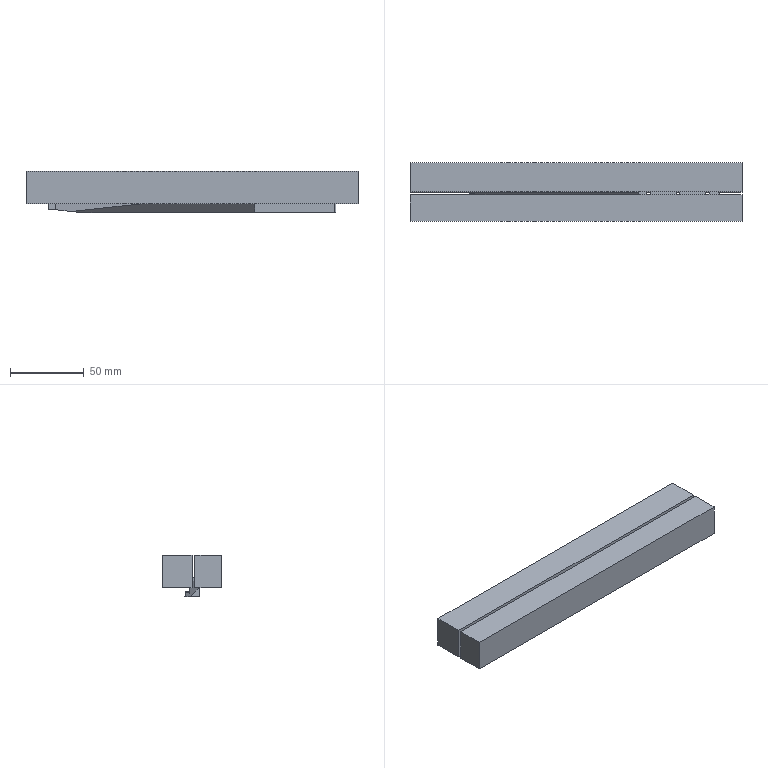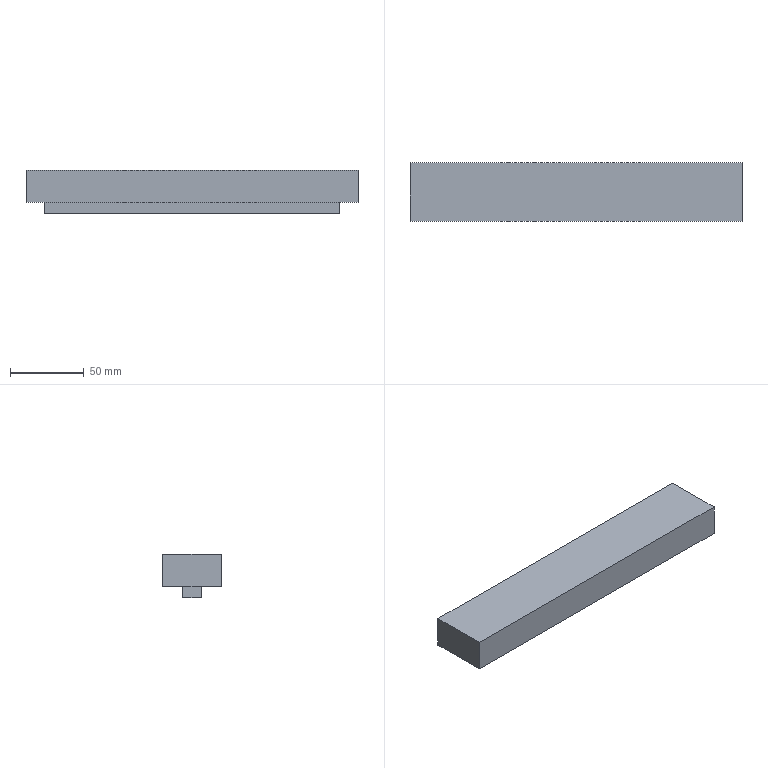CAM job | NX | 3+2 milling, drilling | part box 225.5 x 39.7 x 28 mm | stock box 225.5 x 39.7 x 29.8 mm
Tools:
number,name,description,diameter,corner_radius,flute_length,length,flutes
4,D4,平底铣刀-粗,4.0,0.0,25.0,75.0,2
9,D10,平底铣刀-粗,10.0,0.0,35.0,75.0,2
19,D1.5-J,平底铣刀-粗,1.5,0.0,50.0,75.0,2
17,D2-J,平底铣刀-精,2.0,0.0,50.0,75.0,2
11,D4-J,平底铣刀-精,4.0,0.0,50.0,75.0,2
7,D6-J,平底铣刀-精,6.0,0.0,25.0,75.0,2
18,D4R0.5,圆鼻刀-粗,4.0,0.5,50.0,75.0,2
2,D6倒角刀,倒角刀,6.0,0.0,3.0,25.0,2
20,M3X0.5,丝锥,2.5,0.0,35.0,50.0,2
12,ZT2.5,钻头,2.5,0.0,35.0,50.0,2
Operations:
program,operation,operation_type,tool,method,geometry_group,spindle_rpm,surface_speed,feed_per_tooth,feed_cut,feed_plunge,cut_length_mm,path_length_mm,cut_time_min,machine_time_min
A,底壁铣螺旋开粗-中_COPY,VolumeBased25DMillingOperation,D10,分层开粗-切深K-步距G,W-A,8000.0,251.32,0.25,4000.0,100.0,9915.873,9967.273,2.479,2.484
A,底壁铣分层开粗-中_COPY,VolumeBased25DMillingOperation,D10,分层开粗-切深K-步距G,W-A,8000.0,251.32,0.25,4000.0,100.0,205.014,222.814,0.0513,0.053
A,打点-深0.8_2,Operation,D6倒角刀,NONE,W-A,8000.0,150.796,0.0312,500.0,90.0,5.4,93.45,0.0108,0.0196
A,通孔-M3螺纹底孔_2,Operation,ZT2.5,NONE,W-A,3000.0,23.562,0.05,300.0,90.0,57.453,197.556,0.1915,0.2055
A,钻倒角_1,Operation,D6倒角刀,METHOD,W-A,8000.0,150.796,0.0312,500.0,0.0,14.25,115.547,0.0285,0.0386
A,通孔-攻牙M3_2,Operation,M3X0.5,METHOD,W-A,800.0,6.283,0.0003,0.5,90.0,49.2,181.05,98.4,98.413
A,型腔铣开粗-中_COPY,CavityMilling,D4,分层开粗-切深K-步距G,W-A,8000.0,100.531,0.125,2000.0,100.0,6354.801,6722.452,3.177,3.223
A,底壁铣飞面精光_COPY,VolumeBased25DMillingOperation,D6-J,侧刃精光-切深K-步距G,W-A,8000.0,251.32,0.0625,1000.0,100.0,633.598,669.598,0.6336,0.6372
A,底壁铣精光底面-中_COPY_1,VolumeBased25DMillingOperation,D6-J,精光步距切深关,W-A,7000.0,175.0,0.0536,1500.0,100.0,235.392,254.392,0.1569,0.1588
A,底壁铣精光侧面-中-选底面_COPY,VolumeBased25DMillingOperation,D6-J,侧刃精光-切深K-步距G,W-A,8000.0,150.792,0.0625,1000.0,100.0,21.17,40.17,0.0212,0.0231
A,底壁铣精光侧面-中_COPY,VolumeBased25DMillingOperation,D6-J,侧刃精光-切深K-步距G,W-A,8000.0,150.792,0.0625,1000.0,100.0,1276.651,1321.349,1.277,1.281
A,等高光顺清角D2参考6_COPY,ZLevelMilling,D2-J,分层精光-切深K-步距G,W-A,8000.0,50.264,0.05,800.0,100.0,490.432,536.19,0.613,0.6176
A,曲面D4R2,SurfaceContour,D4R0.5,METHOD,W-A,6000.0,75.0,0.2083,3500.0,100.0,988.904,1023.573,0.2825,0.286
A,曲面D4R2_COPY,SurfaceContour,D4R0.5,METHOD,W-A,6000.0,75.0,0.2083,3500.0,100.0,10183.967,10221.867,2.91,2.913
A,平面去毛刺6X45L_COPY,SurfaceContour,D6倒角刀,爬面_倒角-切深0-步距G,W-A,6500.0,122.519,0.1154,1500.0,100.0,64.161,104.823,0.0428,0.0468
D,底壁挖框-D10_1,VolumeBased25DMillingOperation,D4,METHOD,W-D,8000.0,50.266,0.125,2000.0,100.0,20013.675,20976.633,10.007,10.103
D,等高光顺清角D2参考6_COPY_2,ZLevelMilling,D2-J,分层精光-切深K-步距G,W-D,8000.0,50.264,0.05,800.0,100.0,4043.5,4897.837,5.054,5.14
D,底壁铣精光底面-中_COPY_3,VolumeBased25DMillingOperation,D2-J,精光步距切深关,W-D,7000.0,175.0,0.0536,1500.0,100.0,1292.259,1321.759,0.8615,0.8645
D,等高光顺清角D2参考6_COPY_2_COPY,ZLevelMilling,D1.5-J,分层精光-切深K-步距G,W-D,8000.0,50.264,0.05,800.0,100.0,886.027,1564.048,1.107,1.175
D,平面去毛刺6X45L_COPY_2,SurfaceContour,D6倒角刀,爬面_倒角-切深0-步距G,W-D,6500.0,122.519,0.1154,1500.0,100.0,384.258,521.383,0.2562,0.2699
D,底壁铣精光侧面-中-选底面_COPY_2,VolumeBased25DMillingOperation,D2-J,侧刃精光-切深K-步距G,W-D,8000.0,100.528,0.05,800.0,100.0,1200.105,1231.541,1.5,1.503
B,面铣自动飞面开粗_COPY,FaceMilling,D4,分层开粗-切深K-步距G,W-B,4500.0,890.615,0.3333,3000.0,100.0,5832.45,5992.827,1.944,1.96
B,底壁铣分层开粗-中_COPY_1,VolumeBased25DMillingOperation,D4,分层开粗-切深K-步距G,W-B,8000.0,251.32,0.25,4000.0,100.0,285.745,306.745,0.0714,0.0735
B,型腔铣开粗-中_COPY_1,CavityMilling,D4,分层开粗-切深K-步距G,W-B,8000.0,100.531,0.125,2000.0,100.0,5701.145,6115.71,2.851,2.903
B,面铣自动飞面精光_COPY,FaceMilling,D6-J,侧刃精光-切深K-步距G,W-B,8000.0,150.796,0.0625,1000.0,100.0,640.35,736.35,0.6403,0.6499
B,底壁铣精光底面-中_COPY_1_1,VolumeBased25DMillingOperation,D6-J,精光步距切深关,W-B,7000.0,175.0,0.0536,1500.0,100.0,235.392,256.592,0.1569,0.159
B,底壁铣精光侧面-中-选底面_COPY_1,VolumeBased25DMillingOperation,D6-J,侧刃精光-切深K-步距G,W-B,8000.0,150.792,0.0625,1000.0,100.0,21.17,43.37,0.0212,0.0234
B,等高光顺清角D2参考6_COPY_1,ZLevelMilling,D2-J,分层精光-切深K-步距G,W-B,8000.0,50.264,0.05,800.0,100.0,483.602,589.219,0.6045,0.6151
B,平面去毛刺6X45L_COPY_1,SurfaceContour,D6倒角刀,爬面_倒角-切深0-步距G,W-B,6500.0,122.519,0.1154,1500.0,100.0,64.161,164.823,0.0428,0.0528
B,曲面D4R2_COPY_1,SurfaceContour,D4R0.5,METHOD,W-B,6000.0,75.0,0.2083,3500.0,100.0,1020.928,1116.757,0.2917,0.3013
B,曲面D4R2_COPY_COPY,SurfaceContour,D4R0.5,METHOD,W-B,6000.0,75.0,0.2083,3500.0,100.0,9978.757,10280.251,2.851,2.881
C,底壁挖框-D10,VolumeBased25DMillingOperation,D4,METHOD,W-C,8000.0,100.531,0.125,2000.0,100.0,10240.97,10551.443,5.12,5.152
C,底壁铣精光底面-中_COPY_2,VolumeBased25DMillingOperation,D4-J,精光步距切深关,W-C,7000.0,87.965,0.0714,1000.0,100.0,1578.803,1660.765,1.579,1.587
C,底壁挖框-刀补E6,VolumeBased25DMillingOperation,D4-J,METHOD,W-C,6000.0,75.398,0.0667,800.0,100.0,654.301,1009.879,0.8179,0.8534